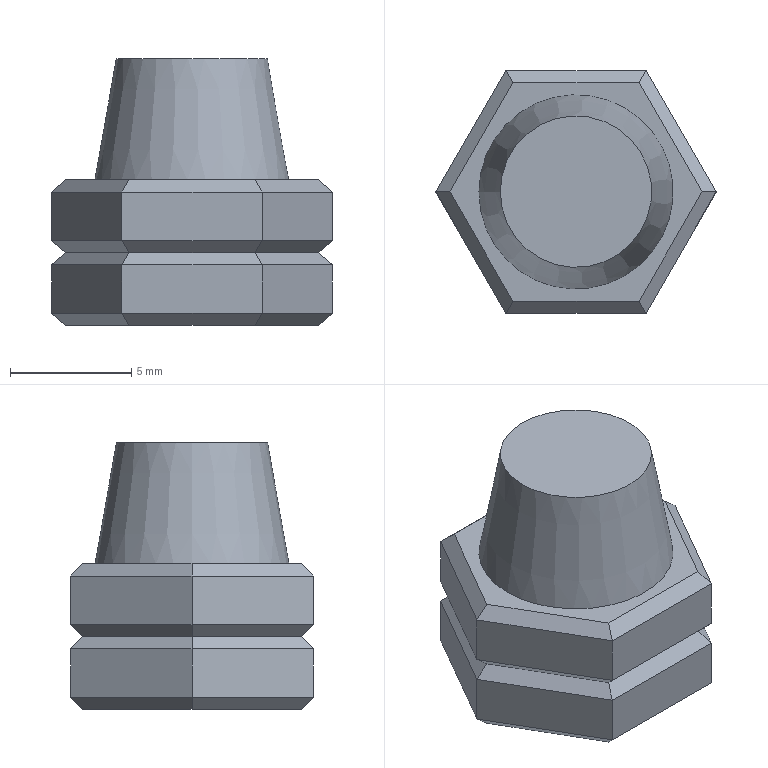Part | STEP file | Tube necking machine_id534_x_t | 1 solid | 40 faces | box 11.547 x 10 x 11 mm | volume 702.875 mm3 | plane 39 | cone 1